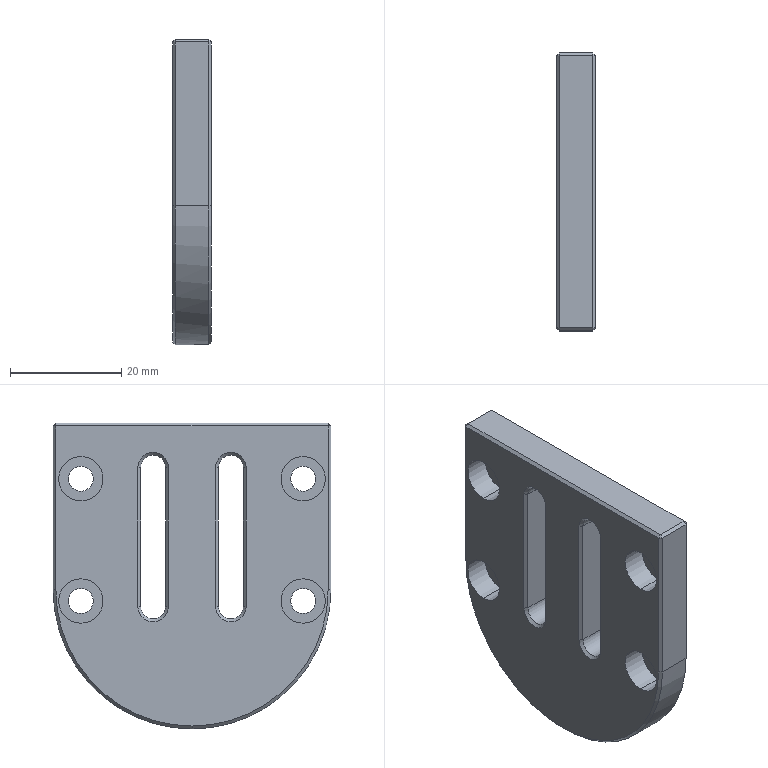Part | STEP file | PN_0015 press block_Default | 1 solid | 71 faces | box 7 x 50 x 55 mm | volume 14443 mm3 | plane 33 | cylinder 23 | cone 15 | commonest cylinder face diameters 4.5 x14 8 x8 50 x1